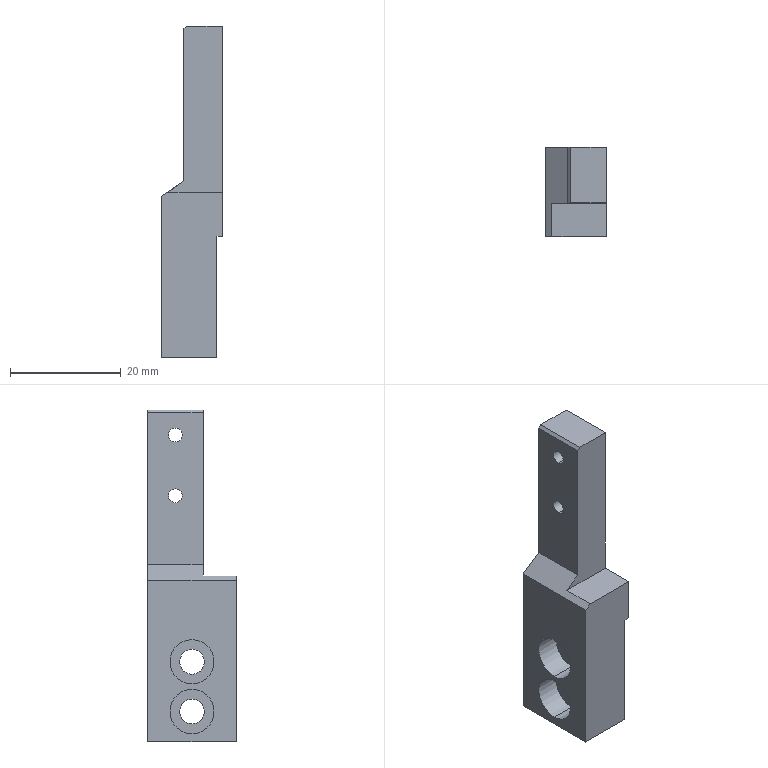Part | SolidWorks | features ICE 7, Chamfer 2, Fillet 2, HoleWzd 2, Cut 1, Extrusion 1 | 1 solid | 33 faces | box 11 x 16 x 60 mm | volume 5664 mm3 | plane 19 | cylinder 14 | commonest cylinder face diameters 2.5 x4 4.5 x4 8 x4 3 x2
STEP:
#1=CARTESIAN_POINT('',(-6.,3.,26.75));
#2=VERTEX_POINT('',#1);
#3=CARTESIAN_POINT('',(-6.,3.,24.25));
#4=VERTEX_POINT('',#3);
#5=CARTESIAN_POINT('',(-6.,3.,25.5));
#6=DIRECTION('',(1.,0.,0.));
#7=DIRECTION('',(0.,0.,-1.));
#8=AXIS2_PLACEMENT_3D('',#5,#6,#7);
#9=CIRCLE('',#8,1.25);
#10=EDGE_CURVE('',#2,#4,#9,.T.);
#11=ORIENTED_EDGE('',*,*,#10,.F.);
#12=CARTESIAN_POINT('',(1.,3.,26.75));
#13=VERTEX_POINT('',#12);
#14=CARTESIAN_POINT('',(1.,3.,26.75));
#15=DIRECTION('',(1.,0.,0.));
#16=VECTOR('',#15,1000.);
#17=LINE('',#14,#16);
#18=EDGE_CURVE('',#2,#13,#17,.T.);
#19=ORIENTED_EDGE('',*,*,#18,.T.);
#20=CARTESIAN_POINT('',(1.,3.,24.25));
#21=VERTEX_POINT('',#20);
#22=CARTESIAN_POINT('',(1.,3.,25.5));
#23=DIRECTION('',(1.,0.,0.));
#24=DIRECTION('',(0.,0.,-1.));
#25=AXIS2_PLACEMENT_3D('',#22,#23,#24);
#26=CIRCLE('',#25,1.25);
#27=EDGE_CURVE('',#13,#21,#26,.T.);
#28=ORIENTED_EDGE('',*,*,#27,.T.);
#29=CARTESIAN_POINT('',(1.,3.,24.25));
#30=DIRECTION('',(1.,0.,0.));
#31=VECTOR('',#30,1000.);
#32=LINE('',#29,#31);
#33=EDGE_CURVE('',#4,#21,#32,.T.);
#34=ORIENTED_EDGE('',*,*,#33,.F.);
#35=EDGE_LOOP('',(#11,#19,#28,#34));
#36=FACE_OUTER_BOUND('',#35,.T.);
#37=CARTESIAN_POINT('',(1.,3.,25.5));
#38=DIRECTION('',(1.,0.,0.));
#39=DIRECTION('',(0.,0.,-1.));
#40=AXIS2_PLACEMENT_3D('',#37,#38,#39);
#41=CYLINDRICAL_SURFACE('',#40,1.25);
#42=ADVANCED_FACE('',(#36),#41,.F.);
#43=CARTESIAN_POINT('',(-6.,3.,15.75));
#44=VERTEX_POINT('',#43);
#45=CARTESIAN_POINT('',(-6.,3.,13.25));
#46=VERTEX_POINT('',#45);
#47=CARTESIAN_POINT('',(-6.,3.,14.5));
#48=DIRECTION('',(1.,0.,0.));
#49=DIRECTION('',(0.,0.,-1.));
#50=AXIS2_PLACEMENT_3D('',#47,#48,#49);
#51=CIRCLE('',#50,1.25);
#52=EDGE_CURVE('',#44,#46,#51,.T.);
#53=ORIENTED_EDGE('',*,*,#52,.F.);
#54=CARTESIAN_POINT('',(1.,3.,15.75));
#55=VERTEX_POINT('',#54);
#56=CARTESIAN_POINT('',(1.,3.,15.75));
#57=DIRECTION('',(1.,0.,0.));
#58=VECTOR('',#57,1000.);
#59=LINE('',#56,#58);
#60=EDGE_CURVE('',#44,#55,#59,.T.);
#61=ORIENTED_EDGE('',*,*,#60,.T.);
#62=CARTESIAN_POINT('',(1.,3.,13.25));
#63=VERTEX_POINT('',#62);
#64=CARTESIAN_POINT('',(1.,3.,14.5));
#65=DIRECTION('',(1.,0.,0.));
#66=DIRECTION('',(0.,0.,-1.));
#67=AXIS2_PLACEMENT_3D('',#64,#65,#66);
#68=CIRCLE('',#67,1.25);
#69=EDGE_CURVE('',#55,#63,#68,.T.);
#70=ORIENTED_EDGE('',*,*,#69,.T.);
#71=CARTESIAN_POINT('',(1.,3.,13.25));
#72=DIRECTION('',(1.,0.,0.));
#73=VECTOR('',#72,1000.);
#74=LINE('',#71,#73);
#75=EDGE_CURVE('',#46,#63,#74,.T.);
#76=ORIENTED_EDGE('',*,*,#75,.F.);
#77=EDGE_LOOP('',(#53,#61,#70,#76));
#78=FACE_OUTER_BOUND('',#77,.T.);
#79=CARTESIAN_POINT('',(1.,3.,14.5));
#80=DIRECTION('',(1.,0.,0.));
#81=DIRECTION('',(0.,0.,-1.));
#82=AXIS2_PLACEMENT_3D('',#79,#80,#81);
#83=CYLINDRICAL_SURFACE('',#82,1.25);
#84=ADVANCED_FACE('',(#78),#83,.F.);
#85=CARTESIAN_POINT('',(-5.6,0.000000653,-19.5));
#86=VERTEX_POINT('',#85);
#87=CARTESIAN_POINT('',(-5.6,0.000000653,-11.5));
#88=VERTEX_POINT('',#87);
#89=CARTESIAN_POINT('',(-5.6,0.000000653,-15.5));
#90=DIRECTION('',(-1.,0.,0.));
#91=DIRECTION('',(0.,0.,1.));
#92=AXIS2_PLACEMENT_3D('',#89,#90,#91);
#93=CIRCLE('',#92,4.);
#94=EDGE_CURVE('',#86,#88,#93,.T.);
#95=ORIENTED_EDGE('',*,*,#94,.F.);
#96=CARTESIAN_POINT('',(-10.,0.000000653,-19.5));
#97=VERTEX_POINT('',#96);
#98=CARTESIAN_POINT('',(-10.,0.000000653,-19.5));
#99=DIRECTION('',(-1.,0.,0.));
#100=VECTOR('',#99,1000.);
#101=LINE('',#98,#100);
#102=EDGE_CURVE('',#86,#97,#101,.T.);
#103=ORIENTED_EDGE('',*,*,#102,.T.);
#104=CARTESIAN_POINT('',(-10.,0.000000653,-11.5));
#105=VERTEX_POINT('',#104);
#106=CARTESIAN_POINT('',(-10.,0.000000653,-15.5));
#107=DIRECTION('',(-1.,0.,0.));
#108=DIRECTION('',(0.,0.,1.));
#109=AXIS2_PLACEMENT_3D('',#106,#107,#108);
#110=CIRCLE('',#109,4.);
#111=EDGE_CURVE('',#97,#105,#110,.T.);
#112=ORIENTED_EDGE('',*,*,#111,.T.);
#113=CARTESIAN_POINT('',(-10.,0.000000653,-11.5));
#114=DIRECTION('',(-1.,0.,0.));
#115=VECTOR('',#114,1000.);
#116=LINE('',#113,#115);
#117=EDGE_CURVE('',#88,#105,#116,.T.);
#118=ORIENTED_EDGE('',*,*,#117,.F.);
#119=EDGE_LOOP('',(#95,#103,#112,#118));
#120=FACE_OUTER_BOUND('',#119,.T.);
#121=CARTESIAN_POINT('',(-10.,0.000000653,-15.5));
#122=DIRECTION('',(-1.,0.,0.));
#123=DIRECTION('',(0.,0.,1.));
#124=AXIS2_PLACEMENT_3D('',#121,#122,#123);
#125=CYLINDRICAL_SURFACE('',#124,4.);
#126=ADVANCED_FACE('',(#120),#125,.F.);
#127=CARTESIAN_POINT('',(-4.,0.000000653,-17.75));
#128=VERTEX_POINT('',#127);
#129=CARTESIAN_POINT('',(-4.,0.000000653,-13.25));
#130=VERTEX_POINT('',#129);
#131=CARTESIAN_POINT('',(-4.,0.000000653,-15.5));
#132=DIRECTION('',(-1.,0.,0.));
#133=DIRECTION('',(0.,0.,1.));
#134=AXIS2_PLACEMENT_3D('',#131,#132,#133);
#135=CIRCLE('',#134,2.25);
#136=EDGE_CURVE('',#128,#130,#135,.T.);
#137=ORIENTED_EDGE('',*,*,#136,.F.);
#138=CARTESIAN_POINT('',(-5.6,0.000000653,-17.75));
#139=VERTEX_POINT('',#138);
#140=CARTESIAN_POINT('',(-10.,0.000000653,-17.75));
#141=DIRECTION('',(-1.,0.,0.));
#142=VECTOR('',#141,1000.);
#143=LINE('',#140,#142);
#144=EDGE_CURVE('',#128,#139,#143,.T.);
#145=ORIENTED_EDGE('',*,*,#144,.T.);
#146=CARTESIAN_POINT('',(-5.6,0.000000653,-13.25));
#147=VERTEX_POINT('',#146);
#148=CARTESIAN_POINT('',(-5.6,0.000000653,-15.5));
#149=DIRECTION('',(-1.,0.,0.));
#150=DIRECTION('',(0.,0.,1.));
#151=AXIS2_PLACEMENT_3D('',#148,#149,#150);
#152=CIRCLE('',#151,2.25);
#153=EDGE_CURVE('',#139,#147,#152,.T.);
#154=ORIENTED_EDGE('',*,*,#153,.T.);
#155=CARTESIAN_POINT('',(-10.,0.000000653,-13.25));
#156=DIRECTION('',(-1.,0.,0.));
#157=VECTOR('',#156,1000.);
#158=LINE('',#155,#157);
#159=EDGE_CURVE('',#130,#147,#158,.T.);
#160=ORIENTED_EDGE('',*,*,#159,.F.);
#161=EDGE_LOOP('',(#137,#145,#154,#160));
#162=FACE_OUTER_BOUND('',#161,.T.);
#163=CARTESIAN_POINT('',(-10.,0.000000653,-15.5));
#164=DIRECTION('',(-1.,0.,0.));
#165=DIRECTION('',(0.,0.,1.));
#166=AXIS2_PLACEMENT_3D('',#163,#164,#165);
#167=CYLINDRICAL_SURFACE('',#166,2.25);
#168=ADVANCED_FACE('',(#162),#167,.F.);
#169=CARTESIAN_POINT('',(-5.6,0.000000653,-28.5));
#170=VERTEX_POINT('',#169);
#171=CARTESIAN_POINT('',(-5.6,0.000000653,-20.5));
#172=VERTEX_POINT('',#171);
#173=CARTESIAN_POINT('',(-5.6,0.000000653,-24.5));
#174=DIRECTION('',(-1.,0.,0.));
#175=DIRECTION('',(0.,0.,1.));
#176=AXIS2_PLACEMENT_3D('',#173,#174,#175);
#177=CIRCLE('',#176,4.);
#178=EDGE_CURVE('',#170,#172,#177,.T.);
#179=ORIENTED_EDGE('',*,*,#178,.F.);
#180=CARTESIAN_POINT('',(-10.,0.000000653,-28.5));
#181=VERTEX_POINT('',#180);
#182=CARTESIAN_POINT('',(-10.,0.000000653,-28.5));
#183=DIRECTION('',(-1.,0.,0.));
#184=VECTOR('',#183,1000.);
#185=LINE('',#182,#184);
#186=EDGE_CURVE('',#170,#181,#185,.T.);
#187=ORIENTED_EDGE('',*,*,#186,.T.);
#188=CARTESIAN_POINT('',(-10.,0.000000653,-20.5));
#189=VERTEX_POINT('',#188);
#190=CARTESIAN_POINT('',(-10.,0.000000653,-24.5));
#191=DIRECTION('',(-1.,0.,0.));
#192=DIRECTION('',(0.,0.,1.));
#193=AXIS2_PLACEMENT_3D('',#190,#191,#192);
#194=CIRCLE('',#193,4.);
#195=EDGE_CURVE('',#181,#189,#194,.T.);
#196=ORIENTED_EDGE('',*,*,#195,.T.);
#197=CARTESIAN_POINT('',(-10.,0.000000653,-20.5));
#198=DIRECTION('',(-1.,0.,0.));
#199=VECTOR('',#198,1000.);
#200=LINE('',#197,#199);
#201=EDGE_CURVE('',#172,#189,#200,.T.);
#202=ORIENTED_EDGE('',*,*,#201,.F.);
#203=EDGE_LOOP('',(#179,#187,#196,#202));
#204=FACE_OUTER_BOUND('',#203,.T.);
#205=CARTESIAN_POINT('',(-10.,0.000000653,-24.5));
#206=DIRECTION('',(-1.,0.,0.));
#207=DIRECTION('',(0.,0.,1.));
#208=AXIS2_PLACEMENT_3D('',#205,#206,#207);
#209=CYLINDRICAL_SURFACE('',#208,4.);
#210=ADVANCED_FACE('',(#204),#209,.F.);
#211=CARTESIAN_POINT('',(-4.,0.000000653,-26.75));
#212=VERTEX_POINT('',#211);
#213=CARTESIAN_POINT('',(-4.,0.000000653,-22.25));
#214=VERTEX_POINT('',#213);
#215=CARTESIAN_POINT('',(-4.,0.000000653,-24.5));
#216=DIRECTION('',(-1.,0.,0.));
#217=DIRECTION('',(0.,0.,1.));
#218=AXIS2_PLACEMENT_3D('',#215,#216,#217);
#219=CIRCLE('',#218,2.25);
#220=EDGE_CURVE('',#212,#214,#219,.T.);
#221=ORIENTED_EDGE('',*,*,#220,.F.);
#222=CARTESIAN_POINT('',(-5.6,0.000000653,-26.75));
#223=VERTEX_POINT('',#222);
#224=CARTESIAN_POINT('',(-10.,0.000000653,-26.75));
#225=DIRECTION('',(-1.,0.,0.));
#226=VECTOR('',#225,1000.);
#227=LINE('',#224,#226);
#228=EDGE_CURVE('',#212,#223,#227,.T.);
#229=ORIENTED_EDGE('',*,*,#228,.T.);
#230=CARTESIAN_POINT('',(-5.6,0.000000653,-22.25));
#231=VERTEX_POINT('',#230);
#232=CARTESIAN_POINT('',(-5.6,0.000000653,-24.5));
#233=DIRECTION('',(-1.,0.,0.));
#234=DIRECTION('',(0.,0.,1.));
#235=AXIS2_PLACEMENT_3D('',#232,#233,#234);
#236=CIRCLE('',#235,2.25);
#237=EDGE_CURVE('',#223,#231,#236,.T.);
#238=ORIENTED_EDGE('',*,*,#237,.T.);
#239=CARTESIAN_POINT('',(-10.,0.000000653,-22.25));
#240=DIRECTION('',(-1.,0.,0.));
#241=VECTOR('',#240,1000.);
#242=LINE('',#239,#241);
#243=EDGE_CURVE('',#214,#231,#242,.T.);
#244=ORIENTED_EDGE('',*,*,#243,.F.);
#245=EDGE_LOOP('',(#221,#229,#238,#244));
#246=FACE_OUTER_BOUND('',#245,.T.);
#247=CARTESIAN_POINT('',(-10.,0.000000653,-24.5));
#248=DIRECTION('',(-1.,0.,0.));
#249=DIRECTION('',(0.,0.,1.));
#250=AXIS2_PLACEMENT_3D('',#247,#248,#249);
#251=CYLINDRICAL_SURFACE('',#250,2.25);
#252=ADVANCED_FACE('',(#246),#251,.F.);
#253=CARTESIAN_POINT('',(-5.5,-2.,30.));
#254=VERTEX_POINT('',#253);
#255=CARTESIAN_POINT('',(1.,-2.,30.));
#256=VERTEX_POINT('',#255);
#257=CARTESIAN_POINT('',(-10.,-2.,30.));
#258=DIRECTION('',(1.,0.,0.));
#259=VECTOR('',#258,1000.);
#260=LINE('',#257,#259);
#261=EDGE_CURVE('',#254,#256,#260,.T.);
#262=ORIENTED_EDGE('',*,*,#261,.T.);
#263=CARTESIAN_POINT('',(1.,8.,30.));
#264=VERTEX_POINT('',#263);
#265=CARTESIAN_POINT('',(1.,8.,30.));
#266=DIRECTION('',(0.,1.,0.));
#267=VECTOR('',#266,1000.);
#268=LINE('',#265,#267);
#269=EDGE_CURVE('',#256,#264,#268,.T.);
#270=ORIENTED_EDGE('',*,*,#269,.T.);
#271=CARTESIAN_POINT('',(-5.5,8.,30.));
#272=VERTEX_POINT('',#271);
#273=CARTESIAN_POINT('',(-10.,8.,30.));
#274=DIRECTION('',(1.,0.,0.));
#275=VECTOR('',#274,1000.);
#276=LINE('',#273,#275);
#277=EDGE_CURVE('',#272,#264,#276,.T.);
#278=ORIENTED_EDGE('',*,*,#277,.F.);
#279=CARTESIAN_POINT('',(-5.5,8.,30.));
#280=DIRECTION('',(0.,-1.,0.));
#281=VECTOR('',#280,1000.);
#282=LINE('',#279,#281);
#283=EDGE_CURVE('',#272,#254,#282,.T.);
#284=ORIENTED_EDGE('',*,*,#283,.T.);
#285=EDGE_LOOP('',(#262,#270,#278,#284));
#286=FACE_OUTER_BOUND('',#285,.T.);
#287=CARTESIAN_POINT('',(-10.,8.,30.));
#288=DIRECTION('',(0.,0.,-1.));
#289=DIRECTION('',(-1.,0.,0.));
#290=AXIS2_PLACEMENT_3D('',#287,#288,#289);
#291=PLANE('',#290);
#292=ADVANCED_FACE('',(#286),#291,.F.);
#293=CARTESIAN_POINT('',(0.,8.,-30.));
#294=VERTEX_POINT('',#293);
#295=CARTESIAN_POINT('',(-10.,8.,-30.));
#296=VERTEX_POINT('',#295);
#297=CARTESIAN_POINT('',(-10.,8.,-30.));
#298=DIRECTION('',(-1.,0.,0.));
#299=VECTOR('',#298,1000.);
#300=LINE('',#297,#299);
#301=EDGE_CURVE('',#294,#296,#300,.T.);
#302=ORIENTED_EDGE('',*,*,#301,.F.);
#303=CARTESIAN_POINT('',(0.,5.,-30.));
#304=VERTEX_POINT('',#303);
#305=CARTESIAN_POINT('',(0.,8.,-30.));
#306=DIRECTION('',(0.,-1.,0.));
#307=VECTOR('',#306,1000.);
#308=LINE('',#305,#307);
#309=EDGE_CURVE('',#294,#304,#308,.T.);
#310=ORIENTED_EDGE('',*,*,#309,.T.);
#311=CARTESIAN_POINT('',(-4.,5.,-30.));
#312=VERTEX_POINT('',#311);
#313=CARTESIAN_POINT('',(-4.,5.,-30.));
#314=DIRECTION('',(1.,0.,0.));
#315=VECTOR('',#314,1000.);
#316=LINE('',#313,#315);
#317=EDGE_CURVE('',#312,#304,#316,.T.);
#318=ORIENTED_EDGE('',*,*,#317,.F.);
#319=CARTESIAN_POINT('',(-4.,-5.,-30.));
#320=VERTEX_POINT('',#319);
#321=CARTESIAN_POINT('',(-4.,5.,-30.));
#322=DIRECTION('',(0.,1.,0.));
#323=VECTOR('',#322,1000.);
#324=LINE('',#321,#323);
#325=EDGE_CURVE('',#320,#312,#324,.T.);
#326=ORIENTED_EDGE('',*,*,#325,.F.);
#327=CARTESIAN_POINT('',(0.,-5.,-30.));
#328=VERTEX_POINT('',#327);
#329=CARTESIAN_POINT('',(-4.,-5.,-30.));
#330=DIRECTION('',(1.,0.,0.));
#331=VECTOR('',#330,1000.);
#332=LINE('',#329,#331);
#333=EDGE_CURVE('',#320,#328,#332,.T.);
#334=ORIENTED_EDGE('',*,*,#333,.T.);
#335=CARTESIAN_POINT('',(0.,-8.,-30.));
#336=VERTEX_POINT('',#335);
#337=CARTESIAN_POINT('',(0.,8.,-30.));
#338=DIRECTION('',(0.,-1.,0.));
#339=VECTOR('',#338,1000.);
#340=LINE('',#337,#339);
#341=EDGE_CURVE('',#328,#336,#340,.T.);
#342=ORIENTED_EDGE('',*,*,#341,.T.);
#343=CARTESIAN_POINT('',(-10.,-8.,-30.));
#344=VERTEX_POINT('',#343);
#345=CARTESIAN_POINT('',(-10.,-8.,-30.));
#346=DIRECTION('',(-1.,0.,0.));
#347=VECTOR('',#346,1000.);
#348=LINE('',#345,#347);
#349=EDGE_CURVE('',#336,#344,#348,.T.);
#350=ORIENTED_EDGE('',*,*,#349,.T.);
#351=CARTESIAN_POINT('',(-10.,8.,-30.));
#352=DIRECTION('',(0.,-1.,0.));
#353=VECTOR('',#352,1000.);
#354=LINE('',#351,#353);
#355=EDGE_CURVE('',#296,#344,#354,.T.);
#356=ORIENTED_EDGE('',*,*,#355,.F.);
#357=EDGE_LOOP('',(#302,#310,#318,#326,#334,#342,#350,#356));
#358=FACE_OUTER_BOUND('',#357,.T.);
#359=CARTESIAN_POINT('',(-10.,8.,-30.));
#360=DIRECTION('',(0.,0.,1.));
#361=DIRECTION('',(1.,0.,0.));
#362=AXIS2_PLACEMENT_3D('',#359,#360,#361);
#363=PLANE('',#362);
#364=ADVANCED_FACE('',(#358),#363,.F.);
#365=CARTESIAN_POINT('',(-10.,0.000000653,-15.5));
#366=DIRECTION('',(-1.,0.,0.));
#367=DIRECTION('',(0.,0.,1.));
#368=AXIS2_PLACEMENT_3D('',#365,#366,#367);
#369=CIRCLE('',#368,4.);
#370=EDGE_CURVE('',#105,#97,#369,.T.);
#371=ORIENTED_EDGE('',*,*,#370,.F.);
#372=ORIENTED_EDGE('',*,*,#111,.F.);
#373=EDGE_LOOP('',(#371,#372));
#374=FACE_BOUND('',#373,.T.);
#375=CARTESIAN_POINT('',(-10.,0.000000653,-24.5));
#376=DIRECTION('',(-1.,0.,0.));
#377=DIRECTION('',(0.,0.,1.));
#378=AXIS2_PLACEMENT_3D('',#375,#376,#377);
#379=CIRCLE('',#378,4.);
#380=EDGE_CURVE('',#189,#181,#379,.T.);
#381=ORIENTED_EDGE('',*,*,#380,.F.);
#382=ORIENTED_EDGE('',*,*,#195,.F.);
#383=EDGE_LOOP('',(#381,#382));
#384=FACE_BOUND('',#383,.T.);
#385=CARTESIAN_POINT('',(-10.,-8.,-0.8008));
#386=VERTEX_POINT('',#385);
#387=CARTESIAN_POINT('',(-10.,-8.,-30.));
#388=DIRECTION('',(0.,0.,1.));
#389=VECTOR('',#388,1000.);
#390=LINE('',#387,#389);
#391=EDGE_CURVE('',#344,#386,#390,.T.);
#392=ORIENTED_EDGE('',*,*,#391,.T.);
#393=CARTESIAN_POINT('',(-10.,8.,-0.8008));
#394=VERTEX_POINT('',#393);
#395=CARTESIAN_POINT('',(-10.,-105.798,-0.8008));
#396=DIRECTION('',(0.,1.,0.));
#397=VECTOR('',#396,1000.);
#398=LINE('',#395,#397);
#399=EDGE_CURVE('',#386,#394,#398,.T.);
#400=ORIENTED_EDGE('',*,*,#399,.T.);
#401=CARTESIAN_POINT('',(-10.,8.,-30.));
#402=DIRECTION('',(0.,0.,1.));
#403=VECTOR('',#402,1000.);
#404=LINE('',#401,#403);
#405=EDGE_CURVE('',#296,#394,#404,.T.);
#406=ORIENTED_EDGE('',*,*,#405,.F.);
#407=ORIENTED_EDGE('',*,*,#355,.T.);
#408=EDGE_LOOP('',(#392,#400,#406,#407));
#409=FACE_OUTER_BOUND('',#408,.T.);
#410=CARTESIAN_POINT('',(-10.,8.,-30.));
#411=DIRECTION('',(1.,0.,0.));
#412=DIRECTION('',(0.,0.,-1.));
#413=AXIS2_PLACEMENT_3D('',#410,#411,#412);
#414=PLANE('',#413);
#415=ADVANCED_FACE('',(#374,#384,#409),#414,.F.);
#416=CARTESIAN_POINT('',(1.,8.,-8.));
#417=VERTEX_POINT('',#416);
#418=CARTESIAN_POINT('',(1.,8.,-15.45));
#419=DIRECTION('',(0.,0.,1.));
#420=VECTOR('',#419,1000.);
#421=LINE('',#418,#420);
#422=EDGE_CURVE('',#417,#264,#421,.T.);
#423=ORIENTED_EDGE('',*,*,#422,.F.);
#424=CARTESIAN_POINT('',(0.,8.,-8.));
#425=VERTEX_POINT('',#424);
#426=CARTESIAN_POINT('',(0.,8.,-8.));
#427=DIRECTION('',(-1.,0.,0.));
#428=VECTOR('',#427,1000.);
#429=LINE('',#426,#428);
#430=EDGE_CURVE('',#417,#425,#429,.T.);
#431=ORIENTED_EDGE('',*,*,#430,.T.);
#432=CARTESIAN_POINT('',(0.,8.,-30.));
#433=DIRECTION('',(0.,0.,-1.));
#434=VECTOR('',#433,1000.);
#435=LINE('',#432,#434);
#436=EDGE_CURVE('',#425,#294,#435,.T.);
#437=ORIENTED_EDGE('',*,*,#436,.T.);
#438=ORIENTED_EDGE('',*,*,#301,.T.);
#439=ORIENTED_EDGE('',*,*,#405,.T.);
#440=CARTESIAN_POINT('',(-6.,8.,2.));
#441=VERTEX_POINT('',#440);
#442=CARTESIAN_POINT('',(-2.914,8.,4.161));
#443=DIRECTION('',(-0.8192,0.,-0.5736));
#444=VECTOR('',#443,1000.);
#445=LINE('',#442,#444);
#446=EDGE_CURVE('',#441,#394,#445,.T.);
#447=ORIENTED_EDGE('',*,*,#446,.F.);
#448=CARTESIAN_POINT('',(-6.,8.,29.5));
#449=VERTEX_POINT('',#448);
#450=CARTESIAN_POINT('',(-6.,8.,0.));
#451=DIRECTION('',(0.,0.,-1.));
#452=VECTOR('',#451,1000.);
#453=LINE('',#450,#452);
#454=EDGE_CURVE('',#449,#441,#453,.T.);
#455=ORIENTED_EDGE('',*,*,#454,.F.);
#456=CARTESIAN_POINT('',(-17.75,8.,17.75));
#457=DIRECTION('',(0.7071,0.,0.7071));
#458=VECTOR('',#457,1000.);
#459=LINE('',#456,#458);
#460=EDGE_CURVE('',#449,#272,#459,.T.);
#461=ORIENTED_EDGE('',*,*,#460,.T.);
#462=ORIENTED_EDGE('',*,*,#277,.T.);
#463=EDGE_LOOP('',(#423,#431,#437,#438,#439,#447,#455,#461,#462));
#464=FACE_OUTER_BOUND('',#463,.T.);
#465=CARTESIAN_POINT('',(0.,8.,0.));
#466=DIRECTION('',(0.,1.,0.));
#467=DIRECTION('',(0.,0.,1.));
#468=AXIS2_PLACEMENT_3D('',#465,#466,#467);
#469=PLANE('',#468);
#470=ADVANCED_FACE('',(#464),#469,.T.);
#471=CARTESIAN_POINT('',(1.,-8.,-8.));
#472=VERTEX_POINT('',#471);
#473=CARTESIAN_POINT('',(0.,-8.,-8.));
#474=VERTEX_POINT('',#473);
#475=CARTESIAN_POINT('',(0.,-8.,-8.));
#476=DIRECTION('',(-1.,0.,0.));
#477=VECTOR('',#476,1000.);
#478=LINE('',#475,#477);
#479=EDGE_CURVE('',#472,#474,#478,.T.);
#480=ORIENTED_EDGE('',*,*,#479,.F.);
#481=CARTESIAN_POINT('',(1.,-8.,0.));
#482=VERTEX_POINT('',#481);
#483=CARTESIAN_POINT('',(1.,-8.,-15.45));
#484=DIRECTION('',(0.,0.,1.));
#485=VECTOR('',#484,1000.);
#486=LINE('',#483,#485);
#487=EDGE_CURVE('',#472,#482,#486,.T.);
#488=ORIENTED_EDGE('',*,*,#487,.T.);
#489=CARTESIAN_POINT('',(-8.856,-8.,0.));
#490=VERTEX_POINT('',#489);
#491=CARTESIAN_POINT('',(-10.,-8.,0.));
#492=DIRECTION('',(1.,0.,0.));
#493=VECTOR('',#492,1000.);
#494=LINE('',#491,#493);
#495=EDGE_CURVE('',#490,#482,#494,.T.);
#496=ORIENTED_EDGE('',*,*,#495,.F.);
#497=CARTESIAN_POINT('',(-2.914,-8.,4.161));
#498=DIRECTION('',(-0.8192,0.,-0.5736));
#499=VECTOR('',#498,1000.);
#500=LINE('',#497,#499);
#501=EDGE_CURVE('',#490,#386,#500,.T.);
#502=ORIENTED_EDGE('',*,*,#501,.T.);
#503=ORIENTED_EDGE('',*,*,#391,.F.);
#504=ORIENTED_EDGE('',*,*,#349,.F.);
#505=CARTESIAN_POINT('',(0.,-8.,-30.));
#506=DIRECTION('',(0.,0.,-1.));
#507=VECTOR('',#506,1000.);
#508=LINE('',#505,#507);
#509=EDGE_CURVE('',#474,#336,#508,.T.);
#510=ORIENTED_EDGE('',*,*,#509,.F.);
#511=EDGE_LOOP('',(#480,#488,#496,#502,#503,#504,#510));
#512=FACE_OUTER_BOUND('',#511,.T.);
#513=CARTESIAN_POINT('',(0.,-8.,0.));
#514=DIRECTION('',(0.,1.,0.));
#515=DIRECTION('',(0.,0.,1.));
#516=AXIS2_PLACEMENT_3D('',#513,#514,#515);
#517=PLANE('',#516);
#518=ADVANCED_FACE('',(#512),#517,.F.);
#519=CARTESIAN_POINT('',(-4.,-5.,-12.));
#520=VERTEX_POINT('',#519);
#521=CARTESIAN_POINT('',(0.,-5.,-12.));
#522=VERTEX_POINT('',#521);
#523=CARTESIAN_POINT('',(-8.243,-5.,-12.));
#524=DIRECTION('',(1.,0.,0.));
#525=VECTOR('',#524,1000.);
#526=LINE('',#523,#525);
#527=EDGE_CURVE('',#520,#522,#526,.T.);
#528=ORIENTED_EDGE('',*,*,#527,.T.);
#529=CARTESIAN_POINT('',(0.,-5.,-30.));
#530=DIRECTION('',(0.,0.,-1.));
#531=VECTOR('',#530,1000.);
#532=LINE('',#529,#531);
#533=EDGE_CURVE('',#522,#328,#532,.T.);
#534=ORIENTED_EDGE('',*,*,#533,.T.);
#535=ORIENTED_EDGE('',*,*,#333,.F.);
#536=CARTESIAN_POINT('',(-4.,-5.,-30.));
#537=DIRECTION('',(0.,0.,-1.));
#538=VECTOR('',#537,1000.);
#539=LINE('',#536,#538);
#540=EDGE_CURVE('',#520,#320,#539,.T.);
#541=ORIENTED_EDGE('',*,*,#540,.F.);
#542=EDGE_LOOP('',(#528,#534,#535,#541));
#543=FACE_OUTER_BOUND('',#542,.T.);
#544=CARTESIAN_POINT('',(-4.,-5.,-30.));
#545=DIRECTION('',(0.,-1.,0.));
#546=DIRECTION('',(0.,0.,-1.));
#547=AXIS2_PLACEMENT_3D('',#544,#545,#546);
#548=PLANE('',#547);
#549=ADVANCED_FACE('',(#543),#548,.F.);
#550=CARTESIAN_POINT('',(-4.,3.5,-10.5));
#551=VERTEX_POINT('',#550);
#552=CARTESIAN_POINT('',(0.,3.5,-10.5));
#553=VERTEX_POINT('',#552);
#554=CARTESIAN_POINT('',(-8.243,3.5,-10.5));
#555=DIRECTION('',(1.,0.,0.));
#556=VECTOR('',#555,1000.);
#557=LINE('',#554,#556);
#558=EDGE_CURVE('',#551,#553,#557,.T.);
#559=ORIENTED_EDGE('',*,*,#558,.T.);
#560=CARTESIAN_POINT('',(0.,-3.5,-10.5));
#561=VERTEX_POINT('',#560);
#562=CARTESIAN_POINT('',(0.,5.,-10.5));
#563=DIRECTION('',(0.,-1.,0.));
#564=VECTOR('',#563,1000.);
#565=LINE('',#562,#564);
#566=EDGE_CURVE('',#553,#561,#565,.T.);
#567=ORIENTED_EDGE('',*,*,#566,.T.);
#568=CARTESIAN_POINT('',(-4.,-3.5,-10.5));
#569=VERTEX_POINT('',#568);
#570=CARTESIAN_POINT('',(-8.243,-3.5,-10.5));
#571=DIRECTION('',(-1.,0.,0.));
#572=VECTOR('',#571,1000.);
#573=LINE('',#570,#572);
#574=EDGE_CURVE('',#561,#569,#573,.T.);
#575=ORIENTED_EDGE('',*,*,#574,.T.);
#576=CARTESIAN_POINT('',(-4.,5.,-10.5));
#577=DIRECTION('',(0.,-1.,0.));
#578=VECTOR('',#577,1000.);
#579=LINE('',#576,#578);
#580=EDGE_CURVE('',#551,#569,#579,.T.);
#581=ORIENTED_EDGE('',*,*,#580,.F.);
#582=EDGE_LOOP('',(#559,#567,#575,#581));
#583=FACE_OUTER_BOUND('',#582,.T.);
#584=CARTESIAN_POINT('',(-4.,5.,-10.5));
#585=DIRECTION('',(0.,0.,1.));
#586=DIRECTION('',(1.,0.,0.));
#587=AXIS2_PLACEMENT_3D('',#584,#585,#586);
#588=PLANE('',#587);
#589=ADVANCED_FACE('',(#583),#588,.F.);
#590=ORIENTED_EDGE('',*,*,#317,.T.);
#591=CARTESIAN_POINT('',(0.,5.,-12.));
#592=VERTEX_POINT('',#591);
#593=CARTESIAN_POINT('',(0.,5.,-30.));
#594=DIRECTION('',(0.,0.,1.));
#595=VECTOR('',#594,1000.);
#596=LINE('',#593,#595);
#597=EDGE_CURVE('',#304,#592,#596,.T.);
#598=ORIENTED_EDGE('',*,*,#597,.T.);
#599=CARTESIAN_POINT('',(-4.,5.,-12.));
#600=VERTEX_POINT('',#599);
#601=CARTESIAN_POINT('',(-8.243,5.,-12.));
#602=DIRECTION('',(-1.,0.,0.));
#603=VECTOR('',#602,1000.);
#604=LINE('',#601,#603);
#605=EDGE_CURVE('',#592,#600,#604,.T.);
#606=ORIENTED_EDGE('',*,*,#605,.T.);
#607=CARTESIAN_POINT('',(-4.,5.,-30.));
#608=DIRECTION('',(0.,0.,1.));
#609=VECTOR('',#608,1000.);
#610=LINE('',#607,#609);
#611=EDGE_CURVE('',#312,#600,#610,.T.);
#612=ORIENTED_EDGE('',*,*,#611,.F.);
#613=EDGE_LOOP('',(#590,#598,#606,#612));
#614=FACE_OUTER_BOUND('',#613,.T.);
#615=CARTESIAN_POINT('',(-4.,5.,-30.));
#616=DIRECTION('',(0.,1.,0.));
#617=DIRECTION('',(0.,0.,1.));
#618=AXIS2_PLACEMENT_3D('',#615,#616,#617);
#619=PLANE('',#618);
#620=ADVANCED_FACE('',(#614),#619,.F.);
#621=CARTESIAN_POINT('',(-4.,0.000000653,-15.5));
#622=DIRECTION('',(-1.,0.,0.));
#623=DIRECTION('',(0.,0.,1.));
#624=AXIS2_PLACEMENT_3D('',#621,#622,#623);
#625=CIRCLE('',#624,2.25);
#626=EDGE_CURVE('',#130,#128,#625,.T.);
#627=ORIENTED_EDGE('',*,*,#626,.T.);
#628=ORIENTED_EDGE('',*,*,#136,.T.);
#629=EDGE_LOOP('',(#627,#628));
#630=FACE_BOUND('',#629,.T.);
#631=CARTESIAN_POINT('',(-4.,0.000000653,-24.5));
#632=DIRECTION('',(-1.,0.,0.));
#633=DIRECTION('',(0.,0.,1.));
#634=AXIS2_PLACEMENT_3D('',#631,#632,#633);
#635=CIRCLE('',#634,2.25);
#636=EDGE_CURVE('',#214,#212,#635,.T.);
#637=ORIENTED_EDGE('',*,*,#636,.T.);
#638=ORIENTED_EDGE('',*,*,#220,.T.);
#639=EDGE_LOOP('',(#637,#638));
#640=FACE_BOUND('',#639,.T.);
#641=CARTESIAN_POINT('',(-4.,-5.,-10.5));
#642=DIRECTION('',(1.,0.,0.));
#643=DIRECTION('',(0.,0.,1.));
#644=AXIS2_PLACEMENT_3D('',#641,#642,#643);
#645=CIRCLE('',#644,1.5);
#646=EDGE_CURVE('',#569,#520,#645,.T.);
#647=ORIENTED_EDGE('',*,*,#646,.T.);
#648=ORIENTED_EDGE('',*,*,#540,.T.);
#649=ORIENTED_EDGE('',*,*,#325,.T.);
#650=ORIENTED_EDGE('',*,*,#611,.T.);
#651=CARTESIAN_POINT('',(-4.,5.,-10.5));
#652=DIRECTION('',(1.,0.,0.));
#653=DIRECTION('',(0.,0.,1.));
#654=AXIS2_PLACEMENT_3D('',#651,#652,#653);
#655=CIRCLE('',#654,1.5);
#656=EDGE_CURVE('',#600,#551,#655,.T.);
#657=ORIENTED_EDGE('',*,*,#656,.T.);
#658=ORIENTED_EDGE('',*,*,#580,.T.);
#659=EDGE_LOOP('',(#647,#648,#649,#650,#657,#658));
#660=FACE_OUTER_BOUND('',#659,.T.);
#661=CARTESIAN_POINT('',(-4.,0.,0.));
#662=DIRECTION('',(-1.,0.,0.));
#663=DIRECTION('',(0.,0.,1.));
#664=AXIS2_PLACEMENT_3D('',#661,#662,#663);
#665=PLANE('',#664);
#666=ADVANCED_FACE('',(#630,#640,#660),#665,.F.);
#667=CARTESIAN_POINT('',(-6.,3.,25.5));
#668=DIRECTION('',(1.,0.,0.));
#669=DIRECTION('',(0.,0.,-1.));
#670=AXIS2_PLACEMENT_3D('',#667,#668,#669);
#671=CIRCLE('',#670,1.25);
#672=EDGE_CURVE('',#4,#2,#671,.T.);
#673=ORIENTED_EDGE('',*,*,#672,.T.);
#674=ORIENTED_EDGE('',*,*,#10,.T.);
#675=EDGE_LOOP('',(#673,#674));
#676=FACE_BOUND('',#675,.T.);
#677=CARTESIAN_POINT('',(-6.,3.,14.5));
#678=DIRECTION('',(1.,0.,0.));
#679=DIRECTION('',(0.,0.,-1.));
#680=AXIS2_PLACEMENT_3D('',#677,#678,#679);
#681=CIRCLE('',#680,1.25);
#682=EDGE_CURVE('',#46,#44,#681,.T.);
#683=ORIENTED_EDGE('',*,*,#682,.T.);
#684=ORIENTED_EDGE('',*,*,#52,.T.);
#685=EDGE_LOOP('',(#683,#684));
#686=FACE_BOUND('',#685,.T.);
#687=CARTESIAN_POINT('',(-6.,-2.,2.));
#688=VERTEX_POINT('',#687);
#689=CARTESIAN_POINT('',(-6.,-105.798,2.));
#690=DIRECTION('',(0.,1.,0.));
#691=VECTOR('',#690,1000.);
#692=LINE('',#689,#691);
#693=EDGE_CURVE('',#688,#441,#692,.T.);
#694=ORIENTED_EDGE('',*,*,#693,.F.);
#695=CARTESIAN_POINT('',(-6.,-2.,29.5));
#696=VERTEX_POINT('',#695);
#697=CARTESIAN_POINT('',(-6.,-2.,30.));
#698=DIRECTION('',(0.,0.,1.));
#699=VECTOR('',#698,1000.);
#700=LINE('',#697,#699);
#701=EDGE_CURVE('',#688,#696,#700,.T.);
#702=ORIENTED_EDGE('',*,*,#701,.T.);
#703=CARTESIAN_POINT('',(-6.,-105.798,29.5));
#704=DIRECTION('',(0.,1.,0.));
#705=VECTOR('',#704,1000.);
#706=LINE('',#703,#705);
#707=EDGE_CURVE('',#696,#449,#706,.T.);
#708=ORIENTED_EDGE('',*,*,#707,.T.);
#709=ORIENTED_EDGE('',*,*,#454,.T.);
#710=EDGE_LOOP('',(#694,#702,#708,#709));
#711=FACE_OUTER_BOUND('',#710,.T.);
#712=CARTESIAN_POINT('',(-6.,-105.798,30.));
#713=DIRECTION('',(1.,0.,0.));
#714=DIRECTION('',(0.,0.,-1.));
#715=AXIS2_PLACEMENT_3D('',#712,#713,#714);
#716=PLANE('',#715);
#717=ADVANCED_FACE('',(#676,#686,#711),#716,.F.);
#718=CARTESIAN_POINT('',(-8.856,-2.,0.));
#719=VERTEX_POINT('',#718);
#720=CARTESIAN_POINT('',(-8.856,-105.798,0.));
#721=DIRECTION('',(0.,1.,0.));
#722=VECTOR('',#721,1000.);
#723=LINE('',#720,#722);
#724=EDGE_CURVE('',#490,#719,#723,.T.);
#725=ORIENTED_EDGE('',*,*,#724,.T.);
#726=CARTESIAN_POINT('',(-6.,-2.,2.));
#727=DIRECTION('',(0.8192,0.,0.5736));
#728=VECTOR('',#727,1000.);
#729=LINE('',#726,#728);
#730=EDGE_CURVE('',#719,#688,#729,.T.);
#731=ORIENTED_EDGE('',*,*,#730,.T.);
#732=ORIENTED_EDGE('',*,*,#693,.T.);
#733=ORIENTED_EDGE('',*,*,#446,.T.);
#734=ORIENTED_EDGE('',*,*,#399,.F.);
#735=ORIENTED_EDGE('',*,*,#501,.F.);
#736=EDGE_LOOP('',(#725,#731,#732,#733,#734,#735));
#737=FACE_OUTER_BOUND('',#736,.T.);
#738=CARTESIAN_POINT('',(-6.,-105.798,2.));
#739=DIRECTION('',(0.5736,0.,-0.8192));
#740=DIRECTION('',(-0.8192,0.,-0.5736));
#741=AXIS2_PLACEMENT_3D('',#738,#739,#740);
#742=PLANE('',#741);
#743=ADVANCED_FACE('',(#737),#742,.F.);
#744=CARTESIAN_POINT('',(-6.,-2.,29.5));
#745=DIRECTION('',(-0.7071,0.,-0.7071));
#746=VECTOR('',#745,1000.);
#747=LINE('',#744,#746);
#748=EDGE_CURVE('',#254,#696,#747,.T.);
#749=ORIENTED_EDGE('',*,*,#748,.F.);
#750=ORIENTED_EDGE('',*,*,#283,.F.);
#751=ORIENTED_EDGE('',*,*,#460,.F.);
#752=ORIENTED_EDGE('',*,*,#707,.F.);
#753=EDGE_LOOP('',(#749,#750,#751,#752));
#754=FACE_OUTER_BOUND('',#753,.T.);
#755=CARTESIAN_POINT('',(-6.,-105.798,29.5));
#756=DIRECTION('',(0.7071,0.,-0.7071));
#757=DIRECTION('',(0.,1.,0.));
#758=AXIS2_PLACEMENT_3D('',#755,#756,#757);
#759=PLANE('',#758);
#760=ADVANCED_FACE('',(#754),#759,.F.);
#761=ORIENTED_EDGE('',*,*,#605,.F.);
#762=CARTESIAN_POINT('',(0.,5.,-10.5));
#763=DIRECTION('',(1.,0.,0.));
#764=DIRECTION('',(0.,0.,1.));
#765=AXIS2_PLACEMENT_3D('',#762,#763,#764);
#766=CIRCLE('',#765,1.5);
#767=EDGE_CURVE('',#592,#553,#766,.T.);
#768=ORIENTED_EDGE('',*,*,#767,.T.);
#769=ORIENTED_EDGE('',*,*,#558,.F.);
#770=ORIENTED_EDGE('',*,*,#656,.F.);
#771=EDGE_LOOP('',(#761,#768,#769,#770));
#772=FACE_OUTER_BOUND('',#771,.T.);
#773=CARTESIAN_POINT('',(-8.243,5.,-10.5));
#774=DIRECTION('',(1.,0.,0.));
#775=DIRECTION('',(0.,0.,-1.));
#776=AXIS2_PLACEMENT_3D('',#773,#774,#775);
#777=CYLINDRICAL_SURFACE('',#776,1.5);
#778=ADVANCED_FACE('',(#772),#777,.F.);
#779=ORIENTED_EDGE('',*,*,#574,.F.);
#780=CARTESIAN_POINT('',(0.,-5.,-10.5));
#781=DIRECTION('',(1.,0.,0.));
#782=DIRECTION('',(0.,0.,1.));
#783=AXIS2_PLACEMENT_3D('',#780,#781,#782);
#784=CIRCLE('',#783,1.5);
#785=EDGE_CURVE('',#561,#522,#784,.T.);
#786=ORIENTED_EDGE('',*,*,#785,.T.);
#787=ORIENTED_EDGE('',*,*,#527,.F.);
#788=ORIENTED_EDGE('',*,*,#646,.F.);
#789=EDGE_LOOP('',(#779,#786,#787,#788));
#790=FACE_OUTER_BOUND('',#789,.T.);
#791=CARTESIAN_POINT('',(-8.243,-5.,-10.5));
#792=DIRECTION('',(1.,0.,0.));
#793=DIRECTION('',(0.,0.,-1.));
#794=AXIS2_PLACEMENT_3D('',#791,#792,#793);
#795=CYLINDRICAL_SURFACE('',#794,1.5);
#796=ADVANCED_FACE('',(#790),#795,.F.);
#797=ORIENTED_EDGE('',*,*,#228,.F.);
#798=ORIENTED_EDGE('',*,*,#636,.F.);
#799=ORIENTED_EDGE('',*,*,#243,.T.);
#800=CARTESIAN_POINT('',(-5.6,0.000000653,-24.5));
#801=DIRECTION('',(-1.,0.,0.));
#802=DIRECTION('',(0.,0.,1.));
#803=AXIS2_PLACEMENT_3D('',#800,#801,#802);
#804=CIRCLE('',#803,2.25);
#805=EDGE_CURVE('',#231,#223,#804,.T.);
#806=ORIENTED_EDGE('',*,*,#805,.T.);
#807=EDGE_LOOP('',(#797,#798,#799,#806));
#808=FACE_OUTER_BOUND('',#807,.T.);
#809=CARTESIAN_POINT('',(-10.,0.000000653,-24.5));
#810=DIRECTION('',(-1.,0.,0.));
#811=DIRECTION('',(0.,0.,1.));
#812=AXIS2_PLACEMENT_3D('',#809,#810,#811);
#813=CYLINDRICAL_SURFACE('',#812,2.25);
#814=ADVANCED_FACE('',(#808),#813,.F.);
#815=ORIENTED_EDGE('',*,*,#805,.F.);
#816=ORIENTED_EDGE('',*,*,#237,.F.);
#817=EDGE_LOOP('',(#815,#816));
#818=FACE_BOUND('',#817,.T.);
#819=CARTESIAN_POINT('',(-5.6,0.000000653,-24.5));
#820=DIRECTION('',(-1.,0.,0.));
#821=DIRECTION('',(0.,0.,1.));
#822=AXIS2_PLACEMENT_3D('',#819,#820,#821);
#823=CIRCLE('',#822,4.);
#824=EDGE_CURVE('',#172,#170,#823,.T.);
#825=ORIENTED_EDGE('',*,*,#824,.T.);
#826=ORIENTED_EDGE('',*,*,#178,.T.);
#827=EDGE_LOOP('',(#825,#826));
#828=FACE_OUTER_BOUND('',#827,.T.);
#829=CARTESIAN_POINT('',(-5.6,2.25,-24.5));
#830=DIRECTION('',(1.,0.,0.));
#831=DIRECTION('',(0.,0.,-1.));
#832=AXIS2_PLACEMENT_3D('',#829,#830,#831);
#833=PLANE('',#832);
#834=ADVANCED_FACE('',(#818,#828),#833,.F.);
#835=ORIENTED_EDGE('',*,*,#186,.F.);
#836=ORIENTED_EDGE('',*,*,#824,.F.);
#837=ORIENTED_EDGE('',*,*,#201,.T.);
#838=ORIENTED_EDGE('',*,*,#380,.T.);
#839=EDGE_LOOP('',(#835,#836,#837,#838));
#840=FACE_OUTER_BOUND('',#839,.T.);
#841=CARTESIAN_POINT('',(-10.,0.000000653,-24.5));
#842=DIRECTION('',(-1.,0.,0.));
#843=DIRECTION('',(0.,0.,1.));
#844=AXIS2_PLACEMENT_3D('',#841,#842,#843);
#845=CYLINDRICAL_SURFACE('',#844,4.);
#846=ADVANCED_FACE('',(#840),#845,.F.);
#847=ORIENTED_EDGE('',*,*,#144,.F.);
#848=ORIENTED_EDGE('',*,*,#626,.F.);
#849=ORIENTED_EDGE('',*,*,#159,.T.);
#850=CARTESIAN_POINT('',(-5.6,0.000000653,-15.5));
#851=DIRECTION('',(-1.,0.,0.));
#852=DIRECTION('',(0.,0.,1.));
#853=AXIS2_PLACEMENT_3D('',#850,#851,#852);
#854=CIRCLE('',#853,2.25);
#855=EDGE_CURVE('',#147,#139,#854,.T.);
#856=ORIENTED_EDGE('',*,*,#855,.T.);
#857=EDGE_LOOP('',(#847,#848,#849,#856));
#858=FACE_OUTER_BOUND('',#857,.T.);
#859=CARTESIAN_POINT('',(-10.,0.000000653,-15.5));
#860=DIRECTION('',(-1.,0.,0.));
#861=DIRECTION('',(0.,0.,1.));
#862=AXIS2_PLACEMENT_3D('',#859,#860,#861);
#863=CYLINDRICAL_SURFACE('',#862,2.25);
#864=ADVANCED_FACE('',(#858),#863,.F.);
#865=ORIENTED_EDGE('',*,*,#855,.F.);
#866=ORIENTED_EDGE('',*,*,#153,.F.);
#867=EDGE_LOOP('',(#865,#866));
#868=FACE_BOUND('',#867,.T.);
#869=CARTESIAN_POINT('',(-5.6,0.000000653,-15.5));
#870=DIRECTION('',(-1.,0.,0.));
#871=DIRECTION('',(0.,0.,1.));
#872=AXIS2_PLACEMENT_3D('',#869,#870,#871);
#873=CIRCLE('',#872,4.);
#874=EDGE_CURVE('',#88,#86,#873,.T.);
#875=ORIENTED_EDGE('',*,*,#874,.T.);
#876=ORIENTED_EDGE('',*,*,#94,.T.);
#877=EDGE_LOOP('',(#875,#876));
#878=FACE_OUTER_BOUND('',#877,.T.);
#879=CARTESIAN_POINT('',(-5.6,2.25,-15.5));
#880=DIRECTION('',(1.,0.,0.));
#881=DIRECTION('',(0.,0.,-1.));
#882=AXIS2_PLACEMENT_3D('',#879,#880,#881);
#883=PLANE('',#882);
#884=ADVANCED_FACE('',(#868,#878),#883,.F.);
#885=ORIENTED_EDGE('',*,*,#102,.F.);
#886=ORIENTED_EDGE('',*,*,#874,.F.);
#887=ORIENTED_EDGE('',*,*,#117,.T.);
#888=ORIENTED_EDGE('',*,*,#370,.T.);
#889=EDGE_LOOP('',(#885,#886,#887,#888));
#890=FACE_OUTER_BOUND('',#889,.T.);
#891=CARTESIAN_POINT('',(-10.,0.000000653,-15.5));
#892=DIRECTION('',(-1.,0.,0.));
#893=DIRECTION('',(0.,0.,1.));
#894=AXIS2_PLACEMENT_3D('',#891,#892,#893);
#895=CYLINDRICAL_SURFACE('',#894,4.);
#896=ADVANCED_FACE('',(#890),#895,.F.);
#897=ORIENTED_EDGE('',*,*,#309,.F.);
#898=ORIENTED_EDGE('',*,*,#436,.F.);
#899=CARTESIAN_POINT('',(0.,8.,-8.));
#900=DIRECTION('',(0.,-1.,0.));
#901=VECTOR('',#900,1000.);
#902=LINE('',#899,#901);
#903=EDGE_CURVE('',#425,#474,#902,.T.);
#904=ORIENTED_EDGE('',*,*,#903,.T.);
#905=ORIENTED_EDGE('',*,*,#509,.T.);
#906=ORIENTED_EDGE('',*,*,#341,.F.);
#907=ORIENTED_EDGE('',*,*,#533,.F.);
#908=ORIENTED_EDGE('',*,*,#785,.F.);
#909=ORIENTED_EDGE('',*,*,#566,.F.);
#910=ORIENTED_EDGE('',*,*,#767,.F.);
#911=ORIENTED_EDGE('',*,*,#597,.F.);
#912=EDGE_LOOP('',(#897,#898,#904,#905,#906,#907,#908,#909,#910,#911));
#913=FACE_OUTER_BOUND('',#912,.T.);
#914=CARTESIAN_POINT('',(0.,8.,-30.));
#915=DIRECTION('',(-1.,0.,0.));
#916=DIRECTION('',(0.,0.,1.));
#917=AXIS2_PLACEMENT_3D('',#914,#915,#916);
#918=PLANE('',#917);
#919=ADVANCED_FACE('',(#913),#918,.F.);
#920=ORIENTED_EDGE('',*,*,#430,.F.);
#921=CARTESIAN_POINT('',(1.,8.,-8.));
#922=DIRECTION('',(0.,-1.,0.));
#923=VECTOR('',#922,1000.);
#924=LINE('',#921,#923);
#925=EDGE_CURVE('',#417,#472,#924,.T.);
#926=ORIENTED_EDGE('',*,*,#925,.T.);
#927=ORIENTED_EDGE('',*,*,#479,.T.);
#928=ORIENTED_EDGE('',*,*,#903,.F.);
#929=EDGE_LOOP('',(#920,#926,#927,#928));
#930=FACE_OUTER_BOUND('',#929,.T.);
#931=CARTESIAN_POINT('',(0.,8.,-8.));
#932=DIRECTION('',(0.,0.,1.));
#933=DIRECTION('',(1.,0.,0.));
#934=AXIS2_PLACEMENT_3D('',#931,#932,#933);
#935=PLANE('',#934);
#936=ADVANCED_FACE('',(#930),#935,.F.);
#937=ORIENTED_EDGE('',*,*,#495,.T.);
#938=CARTESIAN_POINT('',(1.,-2.,0.));
#939=VERTEX_POINT('',#938);
#940=CARTESIAN_POINT('',(1.,-8.,0.));
#941=DIRECTION('',(0.,1.,0.));
#942=VECTOR('',#941,1000.);
#943=LINE('',#940,#942);
#944=EDGE_CURVE('',#482,#939,#943,.T.);
#945=ORIENTED_EDGE('',*,*,#944,.T.);
#946=CARTESIAN_POINT('',(-10.,-2.,0.));
#947=DIRECTION('',(1.,0.,0.));
#948=VECTOR('',#947,1000.);
#949=LINE('',#946,#948);
#950=EDGE_CURVE('',#719,#939,#949,.T.);
#951=ORIENTED_EDGE('',*,*,#950,.F.);
#952=ORIENTED_EDGE('',*,*,#724,.F.);
#953=EDGE_LOOP('',(#937,#945,#951,#952));
#954=FACE_OUTER_BOUND('',#953,.T.);
#955=CARTESIAN_POINT('',(-10.,-8.,0.));
#956=DIRECTION('',(0.,0.,-1.));
#957=DIRECTION('',(-1.,0.,0.));
#958=AXIS2_PLACEMENT_3D('',#955,#956,#957);
#959=PLANE('',#958);
#960=ADVANCED_FACE('',(#954),#959,.F.);
#961=ORIENTED_EDGE('',*,*,#950,.T.);
#962=CARTESIAN_POINT('',(1.,-2.,30.));
#963=DIRECTION('',(0.,0.,1.));
#964=VECTOR('',#963,1000.);
#965=LINE('',#962,#964);
#966=EDGE_CURVE('',#939,#256,#965,.T.);
#967=ORIENTED_EDGE('',*,*,#966,.T.);
#968=ORIENTED_EDGE('',*,*,#261,.F.);
#969=ORIENTED_EDGE('',*,*,#748,.T.);
#970=ORIENTED_EDGE('',*,*,#701,.F.);
#971=ORIENTED_EDGE('',*,*,#730,.F.);
#972=EDGE_LOOP('',(#961,#967,#968,#969,#970,#971));
#973=FACE_OUTER_BOUND('',#972,.T.);
#974=CARTESIAN_POINT('',(-10.,-2.,30.));
#975=DIRECTION('',(0.,1.,0.));
#976=DIRECTION('',(0.,0.,1.));
#977=AXIS2_PLACEMENT_3D('',#974,#975,#976);
#978=PLANE('',#977);
#979=ADVANCED_FACE('',(#973),#978,.F.);
#980=CARTESIAN_POINT('',(1.,3.,25.5));
#981=DIRECTION('',(1.,0.,0.));
#982=DIRECTION('',(0.,0.,-1.));
#983=AXIS2_PLACEMENT_3D('',#980,#981,#982);
#984=CIRCLE('',#983,1.25);
#985=EDGE_CURVE('',#21,#13,#984,.T.);
#986=ORIENTED_EDGE('',*,*,#985,.F.);
#987=ORIENTED_EDGE('',*,*,#27,.F.);
#988=EDGE_LOOP('',(#986,#987));
#989=FACE_BOUND('',#988,.T.);
#990=CARTESIAN_POINT('',(1.,3.,14.5));
#991=DIRECTION('',(1.,0.,0.));
#992=DIRECTION('',(0.,0.,-1.));
#993=AXIS2_PLACEMENT_3D('',#990,#991,#992);
#994=CIRCLE('',#993,1.25);
#995=EDGE_CURVE('',#63,#55,#994,.T.);
#996=ORIENTED_EDGE('',*,*,#995,.F.);
#997=ORIENTED_EDGE('',*,*,#69,.F.);
#998=EDGE_LOOP('',(#996,#997));
#999=FACE_BOUND('',#998,.T.);
#1000=ORIENTED_EDGE('',*,*,#422,.T.);
#1001=ORIENTED_EDGE('',*,*,#269,.F.);
#1002=ORIENTED_EDGE('',*,*,#966,.F.);
#1003=ORIENTED_EDGE('',*,*,#944,.F.);
#1004=ORIENTED_EDGE('',*,*,#487,.F.);
#1005=ORIENTED_EDGE('',*,*,#925,.F.);
#1006=EDGE_LOOP('',(#1000,#1001,#1002,#1003,#1004,#1005));
#1007=FACE_OUTER_BOUND('',#1006,.T.);
#1008=CARTESIAN_POINT('',(1.,-8.,-15.45));
#1009=DIRECTION('',(-1.,0.,0.));
#1010=DIRECTION('',(0.,0.,1.));
#1011=AXIS2_PLACEMENT_3D('',#1008,#1009,#1010);
#1012=PLANE('',#1011);
#1013=ADVANCED_FACE('',(#989,#999,#1007),#1012,.F.);
#1014=ORIENTED_EDGE('',*,*,#60,.F.);
#1015=ORIENTED_EDGE('',*,*,#682,.F.);
#1016=ORIENTED_EDGE('',*,*,#75,.T.);
#1017=ORIENTED_EDGE('',*,*,#995,.T.);
#1018=EDGE_LOOP('',(#1014,#1015,#1016,#1017));
#1019=FACE_OUTER_BOUND('',#1018,.T.);
#1020=CARTESIAN_POINT('',(1.,3.,14.5));
#1021=DIRECTION('',(1.,0.,0.));
#1022=DIRECTION('',(0.,0.,-1.));
#1023=AXIS2_PLACEMENT_3D('',#1020,#1021,#1022);
#1024=CYLINDRICAL_SURFACE('',#1023,1.25);
#1025=ADVANCED_FACE('',(#1019),#1024,.F.);
#1026=ORIENTED_EDGE('',*,*,#18,.F.);
#1027=ORIENTED_EDGE('',*,*,#672,.F.);
#1028=ORIENTED_EDGE('',*,*,#33,.T.);
#1029=ORIENTED_EDGE('',*,*,#985,.T.);
#1030=EDGE_LOOP('',(#1026,#1027,#1028,#1029));
#1031=FACE_OUTER_BOUND('',#1030,.T.);
#1032=CARTESIAN_POINT('',(1.,3.,25.5));
#1033=DIRECTION('',(1.,0.,0.));
#1034=DIRECTION('',(0.,0.,-1.));
#1035=AXIS2_PLACEMENT_3D('',#1032,#1033,#1034);
#1036=CYLINDRICAL_SURFACE('',#1035,1.25);
#1037=ADVANCED_FACE('',(#1031),#1036,.F.);
#1038=CLOSED_SHELL('',(#42,#84,#126,#168,#210,#252,#292,#364,#415,#470,#518,#549,#589,#620,#666,#717,#743,#760,#778,#796,#814,#834,#846,#864,#884,#896,#919,#936,#960,#979,#1013,#1025,#1037));
#1039=MANIFOLD_SOLID_BREP('',#1038);
#1040=CARTESIAN_POINT('',(0.,0.,0.));
#1041=DIRECTION('',(0.,0.,1.));
#1042=DIRECTION('',(1.,0.,0.));
#1043=AXIS2_PLACEMENT_3D('',#1040,#1041,#1042);
#1044=(LENGTH_UNIT()NAMED_UNIT(*)SI_UNIT(.MILLI.,.METRE.));
#1045=UNCERTAINTY_MEASURE_WITH_UNIT(LENGTH_MEASURE(0.00001),#1044,'','');
#1046=(NAMED_UNIT(*)PLANE_ANGLE_UNIT()SI_UNIT($,.RADIAN.));
#1047=(NAMED_UNIT(*)SI_UNIT($,.STERADIAN.)SOLID_ANGLE_UNIT());
#1048=(GEOMETRIC_REPRESENTATION_CONTEXT(3)GLOBAL_UNCERTAINTY_ASSIGNED_CONTEXT((#1045))GLOBAL_UNIT_ASSIGNED_CONTEXT((#1044,#1046,#1047))REPRESENTATION_CONTEXT('',''));
#1049=ADVANCED_BREP_SHAPE_REPRESENTATION('',(#1039,#1043),#1048);